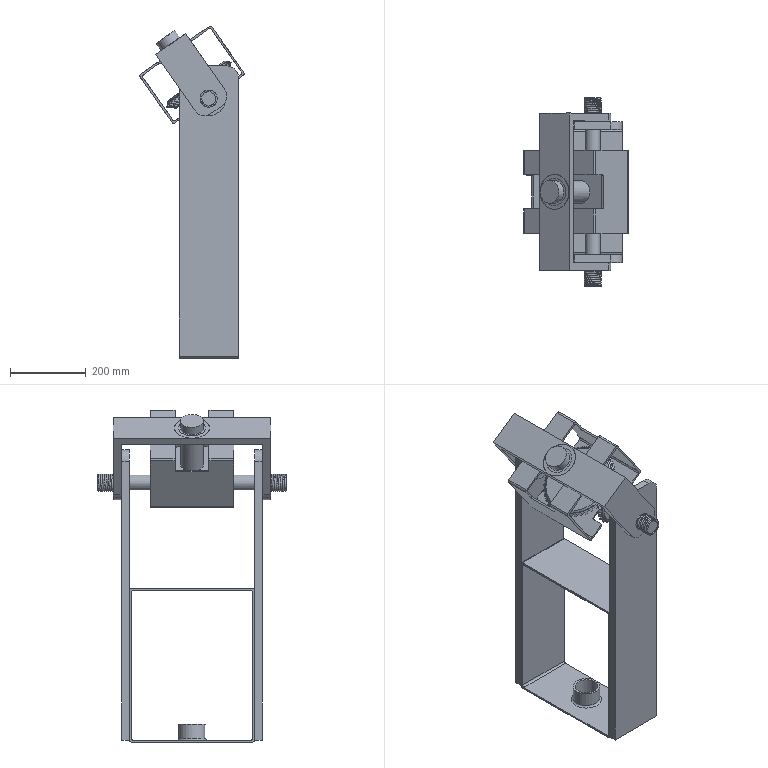Part | NX | features BREP 1 | 18 solids | 1320 faces | box 274.888 x 496 x 875.341 mm | volume 9658258 mm3 | spline 730 | plane 340 | cone 166 | cylinder 80 | torus 4 | commonest cylinder face diameters 10 x40 60 x17 6 x8 40 x5 90 x4 70 x2